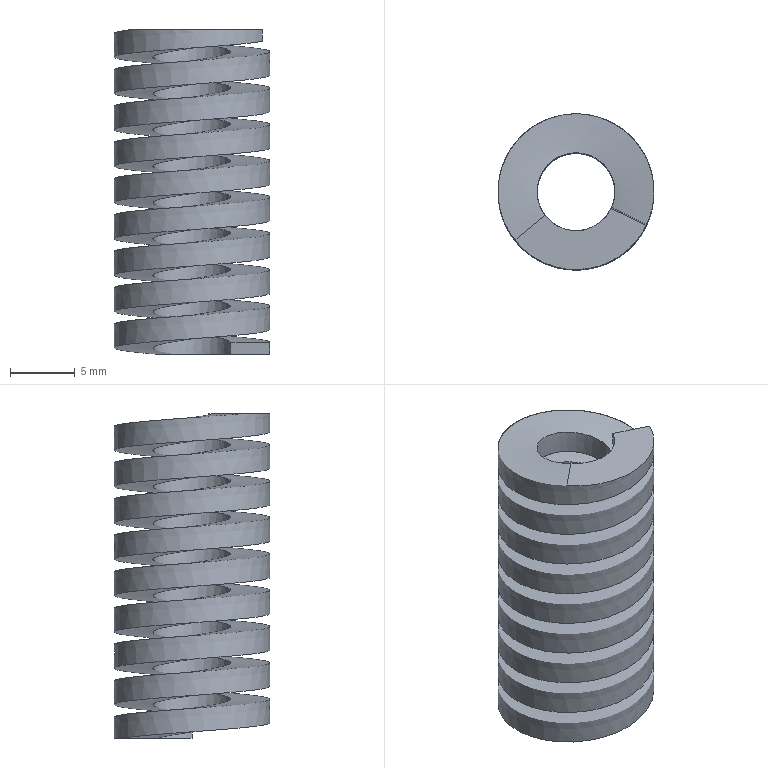Part | STEP file | E011204502 | 1 solid | 6 faces | volume 1367 mm3 | plane 4 | spline 2